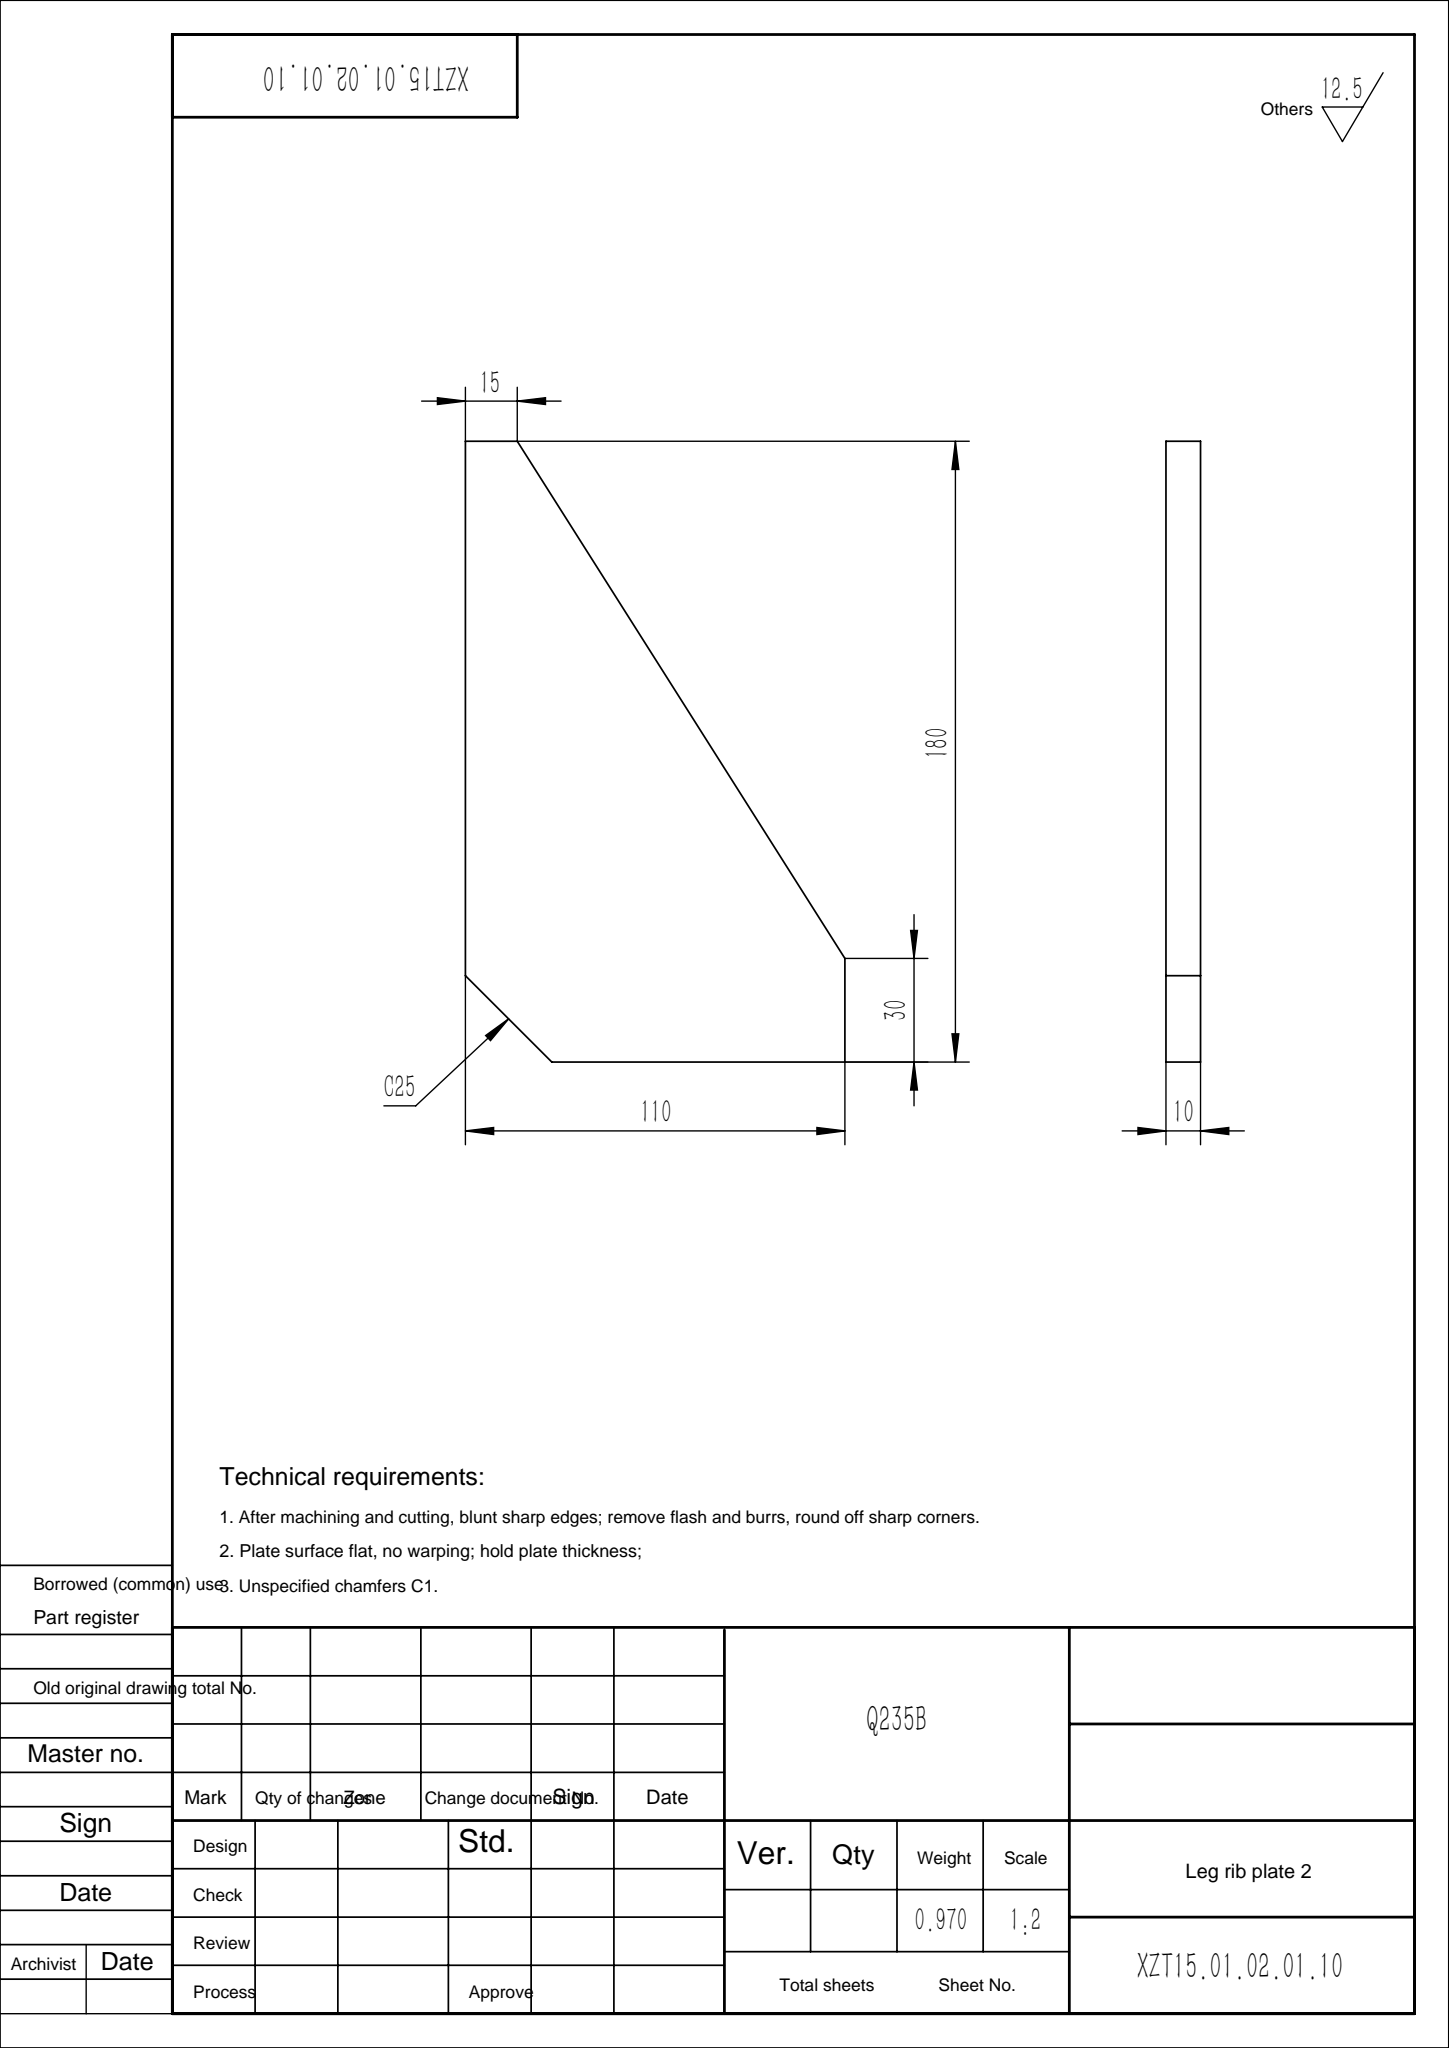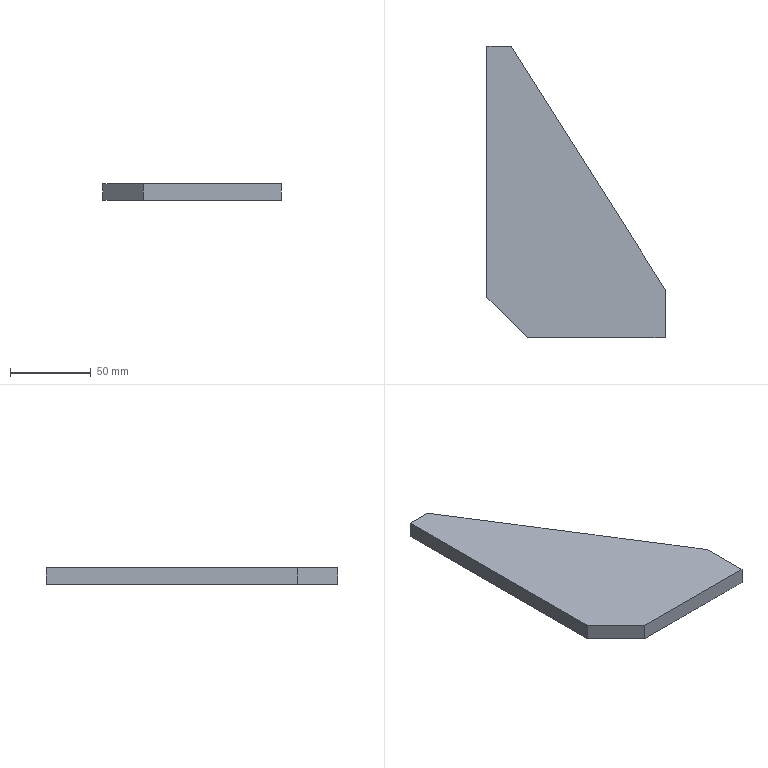Part | SolidWorks | features Chamfer 1, Extrusion 1 | 1 solid | 8 faces | box 110 x 180 x 10 mm | volume 123625 mm3 | plane 8
STEP:
#1=CARTESIAN_POINT('',(0.,180.,-5.));
#2=VERTEX_POINT('',#1);
#3=CARTESIAN_POINT('',(0.,25.,-5.));
#4=VERTEX_POINT('',#3);
#5=CARTESIAN_POINT('',(0.,180.,-5.));
#6=DIRECTION('',(0.,-1.,0.));
#7=VECTOR('',#6,1000.);
#8=LINE('',#5,#7);
#9=EDGE_CURVE('',#2,#4,#8,.T.);
#10=ORIENTED_EDGE('',*,*,#9,.T.);
#11=CARTESIAN_POINT('',(0.,25.,5.));
#12=VERTEX_POINT('',#11);
#13=CARTESIAN_POINT('',(0.,25.,5.));
#14=DIRECTION('',(0.,0.,1.));
#15=VECTOR('',#14,1000.);
#16=LINE('',#13,#15);
#17=EDGE_CURVE('',#4,#12,#16,.T.);
#18=ORIENTED_EDGE('',*,*,#17,.T.);
#19=CARTESIAN_POINT('',(0.,180.,5.));
#20=VERTEX_POINT('',#19);
#21=CARTESIAN_POINT('',(0.,180.,5.));
#22=DIRECTION('',(0.,-1.,0.));
#23=VECTOR('',#22,1000.);
#24=LINE('',#21,#23);
#25=EDGE_CURVE('',#20,#12,#24,.T.);
#26=ORIENTED_EDGE('',*,*,#25,.F.);
#27=CARTESIAN_POINT('',(0.,180.,5.));
#28=DIRECTION('',(0.,0.,-1.));
#29=VECTOR('',#28,1000.);
#30=LINE('',#27,#29);
#31=EDGE_CURVE('',#20,#2,#30,.T.);
#32=ORIENTED_EDGE('',*,*,#31,.T.);
#33=EDGE_LOOP('',(#10,#18,#26,#32));
#34=FACE_OUTER_BOUND('',#33,.T.);
#35=CARTESIAN_POINT('',(0.,180.,5.));
#36=DIRECTION('',(1.,0.,0.));
#37=DIRECTION('',(0.,1.,0.));
#38=AXIS2_PLACEMENT_3D('',#35,#36,#37);
#39=PLANE('',#38);
#40=ADVANCED_FACE('',(#34),#39,.F.);
#41=CARTESIAN_POINT('',(25.,0.,5.));
#42=VERTEX_POINT('',#41);
#43=CARTESIAN_POINT('',(110.,0.,5.));
#44=VERTEX_POINT('',#43);
#45=CARTESIAN_POINT('',(0.,0.,5.));
#46=DIRECTION('',(1.,0.,0.));
#47=VECTOR('',#46,1000.);
#48=LINE('',#45,#47);
#49=EDGE_CURVE('',#42,#44,#48,.T.);
#50=ORIENTED_EDGE('',*,*,#49,.F.);
#51=CARTESIAN_POINT('',(25.,0.,-5.));
#52=VERTEX_POINT('',#51);
#53=CARTESIAN_POINT('',(25.,0.,5.));
#54=DIRECTION('',(0.,0.,-1.));
#55=VECTOR('',#54,1000.);
#56=LINE('',#53,#55);
#57=EDGE_CURVE('',#42,#52,#56,.T.);
#58=ORIENTED_EDGE('',*,*,#57,.T.);
#59=CARTESIAN_POINT('',(110.,0.,-5.));
#60=VERTEX_POINT('',#59);
#61=CARTESIAN_POINT('',(0.,0.,-5.));
#62=DIRECTION('',(1.,0.,0.));
#63=VECTOR('',#62,1000.);
#64=LINE('',#61,#63);
#65=EDGE_CURVE('',#52,#60,#64,.T.);
#66=ORIENTED_EDGE('',*,*,#65,.T.);
#67=CARTESIAN_POINT('',(110.,0.,5.));
#68=DIRECTION('',(0.,0.,-1.));
#69=VECTOR('',#68,1000.);
#70=LINE('',#67,#69);
#71=EDGE_CURVE('',#44,#60,#70,.T.);
#72=ORIENTED_EDGE('',*,*,#71,.F.);
#73=EDGE_LOOP('',(#50,#58,#66,#72));
#74=FACE_OUTER_BOUND('',#73,.T.);
#75=CARTESIAN_POINT('',(0.,0.,5.));
#76=DIRECTION('',(0.,1.,0.));
#77=DIRECTION('',(0.,0.,1.));
#78=AXIS2_PLACEMENT_3D('',#75,#76,#77);
#79=PLANE('',#78);
#80=ADVANCED_FACE('',(#74),#79,.F.);
#81=CARTESIAN_POINT('',(110.,30.,-5.));
#82=VERTEX_POINT('',#81);
#83=CARTESIAN_POINT('',(110.,0.,-5.));
#84=DIRECTION('',(0.,1.,0.));
#85=VECTOR('',#84,1000.);
#86=LINE('',#83,#85);
#87=EDGE_CURVE('',#60,#82,#86,.T.);
#88=ORIENTED_EDGE('',*,*,#87,.T.);
#89=CARTESIAN_POINT('',(110.,30.,5.));
#90=VERTEX_POINT('',#89);
#91=CARTESIAN_POINT('',(110.,30.,5.));
#92=DIRECTION('',(0.,0.,-1.));
#93=VECTOR('',#92,1000.);
#94=LINE('',#91,#93);
#95=EDGE_CURVE('',#90,#82,#94,.T.);
#96=ORIENTED_EDGE('',*,*,#95,.F.);
#97=CARTESIAN_POINT('',(110.,0.,5.));
#98=DIRECTION('',(0.,1.,0.));
#99=VECTOR('',#98,1000.);
#100=LINE('',#97,#99);
#101=EDGE_CURVE('',#44,#90,#100,.T.);
#102=ORIENTED_EDGE('',*,*,#101,.F.);
#103=ORIENTED_EDGE('',*,*,#71,.T.);
#104=EDGE_LOOP('',(#88,#96,#102,#103));
#105=FACE_OUTER_BOUND('',#104,.T.);
#106=CARTESIAN_POINT('',(110.,0.,5.));
#107=DIRECTION('',(-1.,0.,0.));
#108=DIRECTION('',(0.,0.,1.));
#109=AXIS2_PLACEMENT_3D('',#106,#107,#108);
#110=PLANE('',#109);
#111=ADVANCED_FACE('',(#105),#110,.F.);
#112=CARTESIAN_POINT('',(15.,180.,-5.));
#113=VERTEX_POINT('',#112);
#114=CARTESIAN_POINT('',(110.,30.,-5.));
#115=DIRECTION('',(-0.5351,0.8448,0.));
#116=VECTOR('',#115,1000.);
#117=LINE('',#114,#116);
#118=EDGE_CURVE('',#82,#113,#117,.T.);
#119=ORIENTED_EDGE('',*,*,#118,.T.);
#120=CARTESIAN_POINT('',(15.,180.,5.));
#121=VERTEX_POINT('',#120);
#122=CARTESIAN_POINT('',(15.,180.,5.));
#123=DIRECTION('',(0.,0.,-1.));
#124=VECTOR('',#123,1000.);
#125=LINE('',#122,#124);
#126=EDGE_CURVE('',#121,#113,#125,.T.);
#127=ORIENTED_EDGE('',*,*,#126,.F.);
#128=CARTESIAN_POINT('',(110.,30.,5.));
#129=DIRECTION('',(-0.5351,0.8448,0.));
#130=VECTOR('',#129,1000.);
#131=LINE('',#128,#130);
#132=EDGE_CURVE('',#90,#121,#131,.T.);
#133=ORIENTED_EDGE('',*,*,#132,.F.);
#134=ORIENTED_EDGE('',*,*,#95,.T.);
#135=EDGE_LOOP('',(#119,#127,#133,#134));
#136=FACE_OUTER_BOUND('',#135,.T.);
#137=CARTESIAN_POINT('',(110.,30.,5.));
#138=DIRECTION('',(-0.8448,-0.5351,0.));
#139=DIRECTION('',(0.5351,-0.8448,0.));
#140=AXIS2_PLACEMENT_3D('',#137,#138,#139);
#141=PLANE('',#140);
#142=ADVANCED_FACE('',(#136),#141,.F.);
#143=CARTESIAN_POINT('',(15.,180.,-5.));
#144=DIRECTION('',(-1.,0.,0.));
#145=VECTOR('',#144,1000.);
#146=LINE('',#143,#145);
#147=EDGE_CURVE('',#113,#2,#146,.T.);
#148=ORIENTED_EDGE('',*,*,#147,.T.);
#149=ORIENTED_EDGE('',*,*,#31,.F.);
#150=CARTESIAN_POINT('',(15.,180.,5.));
#151=DIRECTION('',(-1.,0.,0.));
#152=VECTOR('',#151,1000.);
#153=LINE('',#150,#152);
#154=EDGE_CURVE('',#121,#20,#153,.T.);
#155=ORIENTED_EDGE('',*,*,#154,.F.);
#156=ORIENTED_EDGE('',*,*,#126,.T.);
#157=EDGE_LOOP('',(#148,#149,#155,#156));
#158=FACE_OUTER_BOUND('',#157,.T.);
#159=CARTESIAN_POINT('',(15.,180.,5.));
#160=DIRECTION('',(0.,-1.,0.));
#161=DIRECTION('',(0.,0.,-1.));
#162=AXIS2_PLACEMENT_3D('',#159,#160,#161);
#163=PLANE('',#162);
#164=ADVANCED_FACE('',(#158),#163,.F.);
#165=ORIENTED_EDGE('',*,*,#25,.T.);
#166=CARTESIAN_POINT('',(12.5,12.5,5.));
#167=DIRECTION('',(0.7071,-0.7071,0.));
#168=VECTOR('',#167,1000.);
#169=LINE('',#166,#168);
#170=EDGE_CURVE('',#12,#42,#169,.T.);
#171=ORIENTED_EDGE('',*,*,#170,.T.);
#172=ORIENTED_EDGE('',*,*,#49,.T.);
#173=ORIENTED_EDGE('',*,*,#101,.T.);
#174=ORIENTED_EDGE('',*,*,#132,.T.);
#175=ORIENTED_EDGE('',*,*,#154,.T.);
#176=EDGE_LOOP('',(#165,#171,#172,#173,#174,#175));
#177=FACE_OUTER_BOUND('',#176,.T.);
#178=CARTESIAN_POINT('',(0.,0.,5.));
#179=DIRECTION('',(0.,0.,1.));
#180=DIRECTION('',(1.,0.,0.));
#181=AXIS2_PLACEMENT_3D('',#178,#179,#180);
#182=PLANE('',#181);
#183=ADVANCED_FACE('',(#177),#182,.T.);
#184=ORIENTED_EDGE('',*,*,#65,.F.);
#185=CARTESIAN_POINT('',(25.,0.,-5.));
#186=DIRECTION('',(-0.7071,0.7071,0.));
#187=VECTOR('',#186,1000.);
#188=LINE('',#185,#187);
#189=EDGE_CURVE('',#52,#4,#188,.T.);
#190=ORIENTED_EDGE('',*,*,#189,.T.);
#191=ORIENTED_EDGE('',*,*,#9,.F.);
#192=ORIENTED_EDGE('',*,*,#147,.F.);
#193=ORIENTED_EDGE('',*,*,#118,.F.);
#194=ORIENTED_EDGE('',*,*,#87,.F.);
#195=EDGE_LOOP('',(#184,#190,#191,#192,#193,#194));
#196=FACE_OUTER_BOUND('',#195,.T.);
#197=CARTESIAN_POINT('',(0.,0.,-5.));
#198=DIRECTION('',(0.,0.,1.));
#199=DIRECTION('',(1.,0.,0.));
#200=AXIS2_PLACEMENT_3D('',#197,#198,#199);
#201=PLANE('',#200);
#202=ADVANCED_FACE('',(#196),#201,.F.);
#203=ORIENTED_EDGE('',*,*,#170,.F.);
#204=ORIENTED_EDGE('',*,*,#17,.F.);
#205=ORIENTED_EDGE('',*,*,#189,.F.);
#206=ORIENTED_EDGE('',*,*,#57,.F.);
#207=EDGE_LOOP('',(#203,#204,#205,#206));
#208=FACE_OUTER_BOUND('',#207,.T.);
#209=CARTESIAN_POINT('',(25.,0.,5.));
#210=DIRECTION('',(0.7071,0.7071,0.));
#211=DIRECTION('',(0.,0.,-1.));
#212=AXIS2_PLACEMENT_3D('',#209,#210,#211);
#213=PLANE('',#212);
#214=ADVANCED_FACE('',(#208),#213,.F.);
#215=CLOSED_SHELL('',(#40,#80,#111,#142,#164,#183,#202,#214));
#216=MANIFOLD_SOLID_BREP('',#215);
#217=CARTESIAN_POINT('',(0.,0.,0.));
#218=DIRECTION('',(0.,0.,1.));
#219=DIRECTION('',(1.,0.,0.));
#220=AXIS2_PLACEMENT_3D('',#217,#218,#219);
#221=(LENGTH_UNIT()NAMED_UNIT(*)SI_UNIT(.MILLI.,.METRE.));
#222=UNCERTAINTY_MEASURE_WITH_UNIT(LENGTH_MEASURE(0.00001),#221,'','');
#223=(NAMED_UNIT(*)PLANE_ANGLE_UNIT()SI_UNIT($,.RADIAN.));
#224=(NAMED_UNIT(*)SI_UNIT($,.STERADIAN.)SOLID_ANGLE_UNIT());
#225=(GEOMETRIC_REPRESENTATION_CONTEXT(3)GLOBAL_UNCERTAINTY_ASSIGNED_CONTEXT((#222))GLOBAL_UNIT_ASSIGNED_CONTEXT((#221,#223,#224))REPRESENTATION_CONTEXT('',''));
#226=ADVANCED_BREP_SHAPE_REPRESENTATION('',(#216,#220),#225);